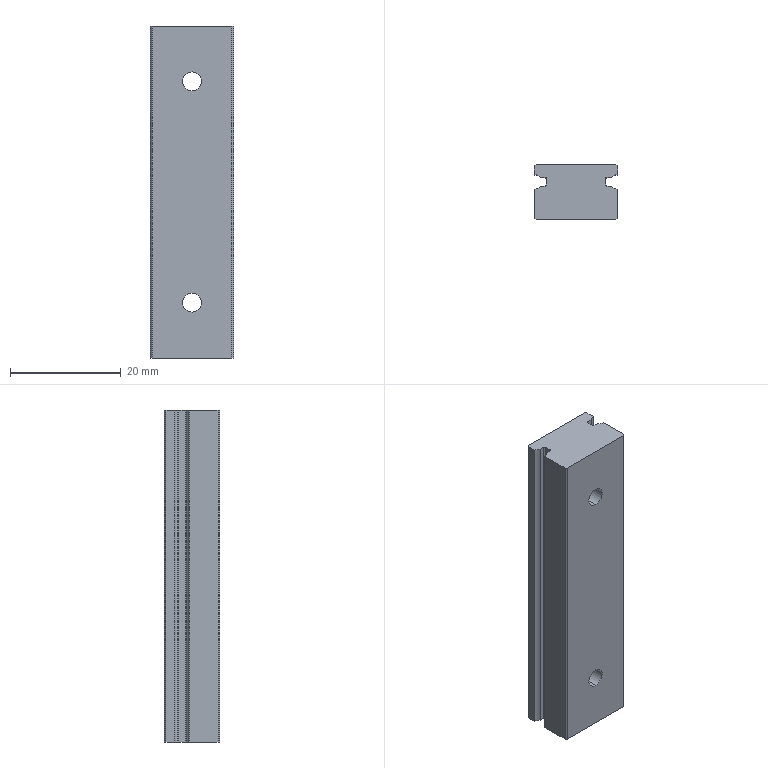Part | SolidWorks | features 3DProfileFeature 1, Extrusion 1, HoleWzd 1, LPattern 1 | 1 solid | 36 faces | box 15 x 10 x 60 mm | volume 8184 mm3 | plane 20 | cylinder 16 | commonest cylinder face diameters 0.4 x4 2.64 x4 3.4 x4 6 x4
STEP:
#1=CARTESIAN_POINT('',(0.,6.6,-23.));
#2=VERTEX_POINT('',#1);
#3=CARTESIAN_POINT('',(0.,6.6,-17.));
#4=VERTEX_POINT('',#3);
#5=CARTESIAN_POINT('',(0.,6.6,-20.));
#6=DIRECTION('',(0.,1.,0.));
#7=DIRECTION('',(0.,0.,1.));
#8=AXIS2_PLACEMENT_3D('',#5,#6,#7);
#9=CIRCLE('',#8,3.);
#10=EDGE_CURVE('',#2,#4,#9,.T.);
#11=ORIENTED_EDGE('',*,*,#10,.F.);
#12=CARTESIAN_POINT('',(0.,10.,-23.));
#13=VERTEX_POINT('',#12);
#14=CARTESIAN_POINT('',(0.,10.,-23.));
#15=DIRECTION('',(0.,1.,0.));
#16=VECTOR('',#15,1000.);
#17=LINE('',#14,#16);
#18=EDGE_CURVE('',#2,#13,#17,.T.);
#19=ORIENTED_EDGE('',*,*,#18,.T.);
#20=CARTESIAN_POINT('',(0.,10.,-17.));
#21=VERTEX_POINT('',#20);
#22=CARTESIAN_POINT('',(0.,10.,-20.));
#23=DIRECTION('',(0.,1.,0.));
#24=DIRECTION('',(0.,0.,1.));
#25=AXIS2_PLACEMENT_3D('',#22,#23,#24);
#26=CIRCLE('',#25,3.);
#27=EDGE_CURVE('',#13,#21,#26,.T.);
#28=ORIENTED_EDGE('',*,*,#27,.T.);
#29=CARTESIAN_POINT('',(0.,10.,-17.));
#30=DIRECTION('',(0.,1.,0.));
#31=VECTOR('',#30,1000.);
#32=LINE('',#29,#31);
#33=EDGE_CURVE('',#4,#21,#32,.T.);
#34=ORIENTED_EDGE('',*,*,#33,.F.);
#35=EDGE_LOOP('',(#11,#19,#28,#34));
#36=FACE_OUTER_BOUND('',#35,.T.);
#37=CARTESIAN_POINT('',(0.,10.,-20.));
#38=DIRECTION('',(0.,1.,0.));
#39=DIRECTION('',(0.,0.,1.));
#40=AXIS2_PLACEMENT_3D('',#37,#38,#39);
#41=CYLINDRICAL_SURFACE('',#40,3.);
#42=ADVANCED_FACE('',(#36),#41,.F.);
#43=CARTESIAN_POINT('',(0.,0.,-21.7));
#44=VERTEX_POINT('',#43);
#45=CARTESIAN_POINT('',(0.,0.,-18.3));
#46=VERTEX_POINT('',#45);
#47=CARTESIAN_POINT('',(0.,0.,-20.));
#48=DIRECTION('',(0.,1.,0.));
#49=DIRECTION('',(0.,0.,1.));
#50=AXIS2_PLACEMENT_3D('',#47,#48,#49);
#51=CIRCLE('',#50,1.7);
#52=EDGE_CURVE('',#44,#46,#51,.T.);
#53=ORIENTED_EDGE('',*,*,#52,.F.);
#54=CARTESIAN_POINT('',(0.,6.6,-21.7));
#55=VERTEX_POINT('',#54);
#56=CARTESIAN_POINT('',(0.,10.,-21.7));
#57=DIRECTION('',(0.,1.,0.));
#58=VECTOR('',#57,1000.);
#59=LINE('',#56,#58);
#60=EDGE_CURVE('',#44,#55,#59,.T.);
#61=ORIENTED_EDGE('',*,*,#60,.T.);
#62=CARTESIAN_POINT('',(0.,6.6,-18.3));
#63=VERTEX_POINT('',#62);
#64=CARTESIAN_POINT('',(0.,6.6,-20.));
#65=DIRECTION('',(0.,1.,0.));
#66=DIRECTION('',(0.,0.,1.));
#67=AXIS2_PLACEMENT_3D('',#64,#65,#66);
#68=CIRCLE('',#67,1.7);
#69=EDGE_CURVE('',#55,#63,#68,.T.);
#70=ORIENTED_EDGE('',*,*,#69,.T.);
#71=CARTESIAN_POINT('',(0.,10.,-18.3));
#72=DIRECTION('',(0.,1.,0.));
#73=VECTOR('',#72,1000.);
#74=LINE('',#71,#73);
#75=EDGE_CURVE('',#46,#63,#74,.T.);
#76=ORIENTED_EDGE('',*,*,#75,.F.);
#77=EDGE_LOOP('',(#53,#61,#70,#76));
#78=FACE_OUTER_BOUND('',#77,.T.);
#79=CARTESIAN_POINT('',(0.,10.,-20.));
#80=DIRECTION('',(0.,1.,0.));
#81=DIRECTION('',(0.,0.,1.));
#82=AXIS2_PLACEMENT_3D('',#79,#80,#81);
#83=CYLINDRICAL_SURFACE('',#82,1.7);
#84=ADVANCED_FACE('',(#78),#83,.F.);
#85=CARTESIAN_POINT('',(0.,6.6,17.));
#86=VERTEX_POINT('',#85);
#87=CARTESIAN_POINT('',(0.,6.6,23.));
#88=VERTEX_POINT('',#87);
#89=CARTESIAN_POINT('',(0.,6.6,20.));
#90=DIRECTION('',(0.,1.,0.));
#91=DIRECTION('',(0.,0.,1.));
#92=AXIS2_PLACEMENT_3D('',#89,#90,#91);
#93=CIRCLE('',#92,3.);
#94=EDGE_CURVE('',#86,#88,#93,.T.);
#95=ORIENTED_EDGE('',*,*,#94,.F.);
#96=CARTESIAN_POINT('',(0.,10.,17.));
#97=VERTEX_POINT('',#96);
#98=CARTESIAN_POINT('',(0.,10.,17.));
#99=DIRECTION('',(0.,1.,0.));
#100=VECTOR('',#99,1000.);
#101=LINE('',#98,#100);
#102=EDGE_CURVE('',#86,#97,#101,.T.);
#103=ORIENTED_EDGE('',*,*,#102,.T.);
#104=CARTESIAN_POINT('',(0.,10.,23.));
#105=VERTEX_POINT('',#104);
#106=CARTESIAN_POINT('',(0.,10.,20.));
#107=DIRECTION('',(0.,1.,0.));
#108=DIRECTION('',(0.,0.,1.));
#109=AXIS2_PLACEMENT_3D('',#106,#107,#108);
#110=CIRCLE('',#109,3.);
#111=EDGE_CURVE('',#97,#105,#110,.T.);
#112=ORIENTED_EDGE('',*,*,#111,.T.);
#113=CARTESIAN_POINT('',(0.,10.,23.));
#114=DIRECTION('',(0.,1.,0.));
#115=VECTOR('',#114,1000.);
#116=LINE('',#113,#115);
#117=EDGE_CURVE('',#88,#105,#116,.T.);
#118=ORIENTED_EDGE('',*,*,#117,.F.);
#119=EDGE_LOOP('',(#95,#103,#112,#118));
#120=FACE_OUTER_BOUND('',#119,.T.);
#121=CARTESIAN_POINT('',(0.,10.,20.));
#122=DIRECTION('',(0.,1.,0.));
#123=DIRECTION('',(0.,0.,1.));
#124=AXIS2_PLACEMENT_3D('',#121,#122,#123);
#125=CYLINDRICAL_SURFACE('',#124,3.);
#126=ADVANCED_FACE('',(#120),#125,.F.);
#127=CARTESIAN_POINT('',(0.,0.,18.3));
#128=VERTEX_POINT('',#127);
#129=CARTESIAN_POINT('',(0.,0.,21.7));
#130=VERTEX_POINT('',#129);
#131=CARTESIAN_POINT('',(0.,0.,20.));
#132=DIRECTION('',(0.,1.,0.));
#133=DIRECTION('',(0.,0.,1.));
#134=AXIS2_PLACEMENT_3D('',#131,#132,#133);
#135=CIRCLE('',#134,1.7);
#136=EDGE_CURVE('',#128,#130,#135,.T.);
#137=ORIENTED_EDGE('',*,*,#136,.F.);
#138=CARTESIAN_POINT('',(0.,6.6,18.3));
#139=VERTEX_POINT('',#138);
#140=CARTESIAN_POINT('',(0.,10.,18.3));
#141=DIRECTION('',(0.,1.,0.));
#142=VECTOR('',#141,1000.);
#143=LINE('',#140,#142);
#144=EDGE_CURVE('',#128,#139,#143,.T.);
#145=ORIENTED_EDGE('',*,*,#144,.T.);
#146=CARTESIAN_POINT('',(0.,6.6,21.7));
#147=VERTEX_POINT('',#146);
#148=CARTESIAN_POINT('',(0.,6.6,20.));
#149=DIRECTION('',(0.,1.,0.));
#150=DIRECTION('',(0.,0.,1.));
#151=AXIS2_PLACEMENT_3D('',#148,#149,#150);
#152=CIRCLE('',#151,1.7);
#153=EDGE_CURVE('',#139,#147,#152,.T.);
#154=ORIENTED_EDGE('',*,*,#153,.T.);
#155=CARTESIAN_POINT('',(0.,10.,21.7));
#156=DIRECTION('',(0.,1.,0.));
#157=VECTOR('',#156,1000.);
#158=LINE('',#155,#157);
#159=EDGE_CURVE('',#130,#147,#158,.T.);
#160=ORIENTED_EDGE('',*,*,#159,.F.);
#161=EDGE_LOOP('',(#137,#145,#154,#160));
#162=FACE_OUTER_BOUND('',#161,.T.);
#163=CARTESIAN_POINT('',(0.,10.,20.));
#164=DIRECTION('',(0.,1.,0.));
#165=DIRECTION('',(0.,0.,1.));
#166=AXIS2_PLACEMENT_3D('',#163,#164,#165);
#167=CYLINDRICAL_SURFACE('',#166,1.7);
#168=ADVANCED_FACE('',(#162),#167,.F.);
#169=CARTESIAN_POINT('',(7.5,8.12,-30.));
#170=VERTEX_POINT('',#169);
#171=CARTESIAN_POINT('',(7.5,9.7,-30.));
#172=VERTEX_POINT('',#171);
#173=CARTESIAN_POINT('',(7.5,8.12,-30.));
#174=DIRECTION('',(0.,1.,0.));
#175=VECTOR('',#174,1000.);
#176=LINE('',#173,#175);
#177=EDGE_CURVE('',#170,#172,#176,.T.);
#178=ORIENTED_EDGE('',*,*,#177,.T.);
#179=CARTESIAN_POINT('',(7.5,9.7,30.));
#180=VERTEX_POINT('',#179);
#181=CARTESIAN_POINT('',(7.5,9.7,30.));
#182=DIRECTION('',(0.,0.,-1.));
#183=VECTOR('',#182,1000.);
#184=LINE('',#181,#183);
#185=EDGE_CURVE('',#180,#172,#184,.T.);
#186=ORIENTED_EDGE('',*,*,#185,.F.);
#187=CARTESIAN_POINT('',(7.5,8.12,30.));
#188=VERTEX_POINT('',#187);
#189=CARTESIAN_POINT('',(7.5,8.12,30.));
#190=DIRECTION('',(0.,1.,0.));
#191=VECTOR('',#190,1000.);
#192=LINE('',#189,#191);
#193=EDGE_CURVE('',#188,#180,#192,.T.);
#194=ORIENTED_EDGE('',*,*,#193,.F.);
#195=CARTESIAN_POINT('',(7.5,8.12,30.));
#196=DIRECTION('',(0.,0.,-1.));
#197=VECTOR('',#196,1000.);
#198=LINE('',#195,#197);
#199=EDGE_CURVE('',#188,#170,#198,.T.);
#200=ORIENTED_EDGE('',*,*,#199,.T.);
#201=EDGE_LOOP('',(#178,#186,#194,#200));
#202=FACE_OUTER_BOUND('',#201,.T.);
#203=CARTESIAN_POINT('',(7.5,8.12,30.));
#204=DIRECTION('',(-1.,0.,0.));
#205=DIRECTION('',(0.,0.,1.));
#206=AXIS2_PLACEMENT_3D('',#203,#204,#205);
#207=PLANE('',#206);
#208=ADVANCED_FACE('',(#202),#207,.F.);
#209=CARTESIAN_POINT('',(7.2,10.,-30.));
#210=VERTEX_POINT('',#209);
#211=CARTESIAN_POINT('',(7.5,9.7,-30.));
#212=DIRECTION('',(-0.7071,0.7071,0.));
#213=VECTOR('',#212,1000.);
#214=LINE('',#211,#213);
#215=EDGE_CURVE('',#172,#210,#214,.T.);
#216=ORIENTED_EDGE('',*,*,#215,.T.);
#217=CARTESIAN_POINT('',(7.2,10.,30.));
#218=VERTEX_POINT('',#217);
#219=CARTESIAN_POINT('',(7.2,10.,30.));
#220=DIRECTION('',(0.,0.,-1.));
#221=VECTOR('',#220,1000.);
#222=LINE('',#219,#221);
#223=EDGE_CURVE('',#218,#210,#222,.T.);
#224=ORIENTED_EDGE('',*,*,#223,.F.);
#225=CARTESIAN_POINT('',(7.5,9.7,30.));
#226=DIRECTION('',(-0.7071,0.7071,0.));
#227=VECTOR('',#226,1000.);
#228=LINE('',#225,#227);
#229=EDGE_CURVE('',#180,#218,#228,.T.);
#230=ORIENTED_EDGE('',*,*,#229,.F.);
#231=ORIENTED_EDGE('',*,*,#185,.T.);
#232=EDGE_LOOP('',(#216,#224,#230,#231));
#233=FACE_OUTER_BOUND('',#232,.T.);
#234=CARTESIAN_POINT('',(7.5,9.7,30.));
#235=DIRECTION('',(-0.7071,-0.7071,0.));
#236=DIRECTION('',(0.7071,-0.7071,0.));
#237=AXIS2_PLACEMENT_3D('',#234,#235,#236);
#238=PLANE('',#237);
#239=ADVANCED_FACE('',(#233),#238,.F.);
#240=CARTESIAN_POINT('',(0.,10.,-20.));
#241=DIRECTION('',(0.,1.,0.));
#242=DIRECTION('',(0.,0.,1.));
#243=AXIS2_PLACEMENT_3D('',#240,#241,#242);
#244=CIRCLE('',#243,3.);
#245=EDGE_CURVE('',#21,#13,#244,.T.);
#246=ORIENTED_EDGE('',*,*,#245,.F.);
#247=ORIENTED_EDGE('',*,*,#27,.F.);
#248=EDGE_LOOP('',(#246,#247));
#249=FACE_BOUND('',#248,.T.);
#250=CARTESIAN_POINT('',(0.,10.,20.));
#251=DIRECTION('',(0.,1.,0.));
#252=DIRECTION('',(0.,0.,1.));
#253=AXIS2_PLACEMENT_3D('',#250,#251,#252);
#254=CIRCLE('',#253,3.);
#255=EDGE_CURVE('',#105,#97,#254,.T.);
#256=ORIENTED_EDGE('',*,*,#255,.F.);
#257=ORIENTED_EDGE('',*,*,#111,.F.);
#258=EDGE_LOOP('',(#256,#257));
#259=FACE_BOUND('',#258,.T.);
#260=CARTESIAN_POINT('',(-7.2,10.,-30.));
#261=VERTEX_POINT('',#260);
#262=CARTESIAN_POINT('',(7.2,10.,-30.));
#263=DIRECTION('',(-1.,0.,0.));
#264=VECTOR('',#263,1000.);
#265=LINE('',#262,#264);
#266=EDGE_CURVE('',#210,#261,#265,.T.);
#267=ORIENTED_EDGE('',*,*,#266,.T.);
#268=CARTESIAN_POINT('',(-7.2,10.,30.));
#269=VERTEX_POINT('',#268);
#270=CARTESIAN_POINT('',(-7.2,10.,30.));
#271=DIRECTION('',(0.,0.,-1.));
#272=VECTOR('',#271,1000.);
#273=LINE('',#270,#272);
#274=EDGE_CURVE('',#269,#261,#273,.T.);
#275=ORIENTED_EDGE('',*,*,#274,.F.);
#276=CARTESIAN_POINT('',(7.2,10.,30.));
#277=DIRECTION('',(-1.,0.,0.));
#278=VECTOR('',#277,1000.);
#279=LINE('',#276,#278);
#280=EDGE_CURVE('',#218,#269,#279,.T.);
#281=ORIENTED_EDGE('',*,*,#280,.F.);
#282=ORIENTED_EDGE('',*,*,#223,.T.);
#283=EDGE_LOOP('',(#267,#275,#281,#282));
#284=FACE_OUTER_BOUND('',#283,.T.);
#285=CARTESIAN_POINT('',(7.2,10.,30.));
#286=DIRECTION('',(0.,-1.,0.));
#287=DIRECTION('',(0.,0.,-1.));
#288=AXIS2_PLACEMENT_3D('',#285,#286,#287);
#289=PLANE('',#288);
#290=ADVANCED_FACE('',(#249,#259,#284),#289,.F.);
#291=CARTESIAN_POINT('',(-7.5,9.7,-30.));
#292=VERTEX_POINT('',#291);
#293=CARTESIAN_POINT('',(-7.2,10.,-30.));
#294=DIRECTION('',(-0.7071,-0.7071,0.));
#295=VECTOR('',#294,1000.);
#296=LINE('',#293,#295);
#297=EDGE_CURVE('',#261,#292,#296,.T.);
#298=ORIENTED_EDGE('',*,*,#297,.T.);
#299=CARTESIAN_POINT('',(-7.5,9.7,30.));
#300=VERTEX_POINT('',#299);
#301=CARTESIAN_POINT('',(-7.5,9.7,30.));
#302=DIRECTION('',(0.,0.,-1.));
#303=VECTOR('',#302,1000.);
#304=LINE('',#301,#303);
#305=EDGE_CURVE('',#300,#292,#304,.T.);
#306=ORIENTED_EDGE('',*,*,#305,.F.);
#307=CARTESIAN_POINT('',(-7.2,10.,30.));
#308=DIRECTION('',(-0.7071,-0.7071,0.));
#309=VECTOR('',#308,1000.);
#310=LINE('',#307,#309);
#311=EDGE_CURVE('',#269,#300,#310,.T.);
#312=ORIENTED_EDGE('',*,*,#311,.F.);
#313=ORIENTED_EDGE('',*,*,#274,.T.);
#314=EDGE_LOOP('',(#298,#306,#312,#313));
#315=FACE_OUTER_BOUND('',#314,.T.);
#316=CARTESIAN_POINT('',(-7.2,10.,30.));
#317=DIRECTION('',(0.7071,-0.7071,0.));
#318=DIRECTION('',(0.7071,0.7071,0.));
#319=AXIS2_PLACEMENT_3D('',#316,#317,#318);
#320=PLANE('',#319);
#321=ADVANCED_FACE('',(#315),#320,.F.);
#322=CARTESIAN_POINT('',(-7.5,8.12,-30.));
#323=VERTEX_POINT('',#322);
#324=CARTESIAN_POINT('',(-7.5,9.7,-30.));
#325=DIRECTION('',(0.,-1.,0.));
#326=VECTOR('',#325,1000.);
#327=LINE('',#324,#326);
#328=EDGE_CURVE('',#292,#323,#327,.T.);
#329=ORIENTED_EDGE('',*,*,#328,.T.);
#330=CARTESIAN_POINT('',(-7.5,8.12,30.));
#331=VERTEX_POINT('',#330);
#332=CARTESIAN_POINT('',(-7.5,8.12,30.));
#333=DIRECTION('',(0.,0.,-1.));
#334=VECTOR('',#333,1000.);
#335=LINE('',#332,#334);
#336=EDGE_CURVE('',#331,#323,#335,.T.);
#337=ORIENTED_EDGE('',*,*,#336,.F.);
#338=CARTESIAN_POINT('',(-7.5,9.7,30.));
#339=DIRECTION('',(0.,-1.,0.));
#340=VECTOR('',#339,1000.);
#341=LINE('',#338,#340);
#342=EDGE_CURVE('',#300,#331,#341,.T.);
#343=ORIENTED_EDGE('',*,*,#342,.F.);
#344=ORIENTED_EDGE('',*,*,#305,.T.);
#345=EDGE_LOOP('',(#329,#337,#343,#344));
#346=FACE_OUTER_BOUND('',#345,.T.);
#347=CARTESIAN_POINT('',(-7.5,9.7,30.));
#348=DIRECTION('',(1.,0.,0.));
#349=DIRECTION('',(0.,0.,-1.));
#350=AXIS2_PLACEMENT_3D('',#347,#348,#349);
#351=PLANE('',#350);
#352=ADVANCED_FACE('',(#346),#351,.F.);
#353=CARTESIAN_POINT('',(-6.45,7.6,-30.));
#354=VERTEX_POINT('',#353);
#355=CARTESIAN_POINT('',(-7.5,6.8,-30.));
#356=DIRECTION('',(0.,0.,-1.));
#357=DIRECTION('',(1.,0.,0.));
#358=AXIS2_PLACEMENT_3D('',#355,#356,#357);
#359=CIRCLE('',#358,1.32);
#360=EDGE_CURVE('',#323,#354,#359,.T.);
#361=ORIENTED_EDGE('',*,*,#360,.T.);
#362=CARTESIAN_POINT('',(-6.45,7.6,30.));
#363=VERTEX_POINT('',#362);
#364=CARTESIAN_POINT('',(-6.45,7.6,30.));
#365=DIRECTION('',(0.,0.,-1.));
#366=VECTOR('',#365,1000.);
#367=LINE('',#364,#366);
#368=EDGE_CURVE('',#363,#354,#367,.T.);
#369=ORIENTED_EDGE('',*,*,#368,.F.);
#370=CARTESIAN_POINT('',(-7.5,6.8,30.));
#371=DIRECTION('',(0.,0.,-1.));
#372=DIRECTION('',(1.,0.,0.));
#373=AXIS2_PLACEMENT_3D('',#370,#371,#372);
#374=CIRCLE('',#373,1.32);
#375=EDGE_CURVE('',#331,#363,#374,.T.);
#376=ORIENTED_EDGE('',*,*,#375,.F.);
#377=ORIENTED_EDGE('',*,*,#336,.T.);
#378=EDGE_LOOP('',(#361,#369,#376,#377));
#379=FACE_OUTER_BOUND('',#378,.T.);
#380=CARTESIAN_POINT('',(-7.5,6.8,30.));
#381=DIRECTION('',(0.,0.,-1.));
#382=DIRECTION('',(-1.,0.,0.));
#383=AXIS2_PLACEMENT_3D('',#380,#381,#382);
#384=CYLINDRICAL_SURFACE('',#383,1.32);
#385=ADVANCED_FACE('',(#379),#384,.F.);
#386=CARTESIAN_POINT('',(-5.6,7.6,-30.));
#387=VERTEX_POINT('',#386);
#388=CARTESIAN_POINT('',(-6.45,7.6,-30.));
#389=DIRECTION('',(1.,0.,0.));
#390=VECTOR('',#389,1000.);
#391=LINE('',#388,#390);
#392=EDGE_CURVE('',#354,#387,#391,.T.);
#393=ORIENTED_EDGE('',*,*,#392,.T.);
#394=CARTESIAN_POINT('',(-5.6,7.6,30.));
#395=VERTEX_POINT('',#394);
#396=CARTESIAN_POINT('',(-5.6,7.6,30.));
#397=DIRECTION('',(0.,0.,-1.));
#398=VECTOR('',#397,1000.);
#399=LINE('',#396,#398);
#400=EDGE_CURVE('',#395,#387,#399,.T.);
#401=ORIENTED_EDGE('',*,*,#400,.F.);
#402=CARTESIAN_POINT('',(-6.45,7.6,30.));
#403=DIRECTION('',(1.,0.,0.));
#404=VECTOR('',#403,1000.);
#405=LINE('',#402,#404);
#406=EDGE_CURVE('',#363,#395,#405,.T.);
#407=ORIENTED_EDGE('',*,*,#406,.F.);
#408=ORIENTED_EDGE('',*,*,#368,.T.);
#409=EDGE_LOOP('',(#393,#401,#407,#408));
#410=FACE_OUTER_BOUND('',#409,.T.);
#411=CARTESIAN_POINT('',(-6.45,7.6,30.));
#412=DIRECTION('',(0.,1.,0.));
#413=DIRECTION('',(0.,0.,1.));
#414=AXIS2_PLACEMENT_3D('',#411,#412,#413);
#415=PLANE('',#414);
#416=ADVANCED_FACE('',(#410),#415,.F.);
#417=CARTESIAN_POINT('',(-5.4,7.4,-30.));
#418=VERTEX_POINT('',#417);
#419=CARTESIAN_POINT('',(-5.6,7.4,-30.));
#420=DIRECTION('',(0.,0.,-1.));
#421=DIRECTION('',(1.,0.,0.));
#422=AXIS2_PLACEMENT_3D('',#419,#420,#421);
#423=CIRCLE('',#422,0.2);
#424=EDGE_CURVE('',#387,#418,#423,.T.);
#425=ORIENTED_EDGE('',*,*,#424,.T.);
#426=CARTESIAN_POINT('',(-5.4,7.4,30.));
#427=VERTEX_POINT('',#426);
#428=CARTESIAN_POINT('',(-5.4,7.4,30.));
#429=DIRECTION('',(0.,0.,-1.));
#430=VECTOR('',#429,1000.);
#431=LINE('',#428,#430);
#432=EDGE_CURVE('',#427,#418,#431,.T.);
#433=ORIENTED_EDGE('',*,*,#432,.F.);
#434=CARTESIAN_POINT('',(-5.6,7.4,30.));
#435=DIRECTION('',(0.,0.,-1.));
#436=DIRECTION('',(1.,0.,0.));
#437=AXIS2_PLACEMENT_3D('',#434,#435,#436);
#438=CIRCLE('',#437,0.2);
#439=EDGE_CURVE('',#395,#427,#438,.T.);
#440=ORIENTED_EDGE('',*,*,#439,.F.);
#441=ORIENTED_EDGE('',*,*,#400,.T.);
#442=EDGE_LOOP('',(#425,#433,#440,#441));
#443=FACE_OUTER_BOUND('',#442,.T.);
#444=CARTESIAN_POINT('',(-5.6,7.4,30.));
#445=DIRECTION('',(0.,0.,-1.));
#446=DIRECTION('',(-1.,0.,0.));
#447=AXIS2_PLACEMENT_3D('',#444,#445,#446);
#448=CYLINDRICAL_SURFACE('',#447,0.2);
#449=ADVANCED_FACE('',(#443),#448,.F.);
#450=CARTESIAN_POINT('',(-5.4,6.2,-30.));
#451=VERTEX_POINT('',#450);
#452=CARTESIAN_POINT('',(-5.4,7.4,-30.));
#453=DIRECTION('',(0.,-1.,0.));
#454=VECTOR('',#453,1000.);
#455=LINE('',#452,#454);
#456=EDGE_CURVE('',#418,#451,#455,.T.);
#457=ORIENTED_EDGE('',*,*,#456,.T.);
#458=CARTESIAN_POINT('',(-5.4,6.2,30.));
#459=VERTEX_POINT('',#458);
#460=CARTESIAN_POINT('',(-5.4,6.2,30.));
#461=DIRECTION('',(0.,0.,-1.));
#462=VECTOR('',#461,1000.);
#463=LINE('',#460,#462);
#464=EDGE_CURVE('',#459,#451,#463,.T.);
#465=ORIENTED_EDGE('',*,*,#464,.F.);
#466=CARTESIAN_POINT('',(-5.4,7.4,30.));
#467=DIRECTION('',(0.,-1.,0.));
#468=VECTOR('',#467,1000.);
#469=LINE('',#466,#468);
#470=EDGE_CURVE('',#427,#459,#469,.T.);
#471=ORIENTED_EDGE('',*,*,#470,.F.);
#472=ORIENTED_EDGE('',*,*,#432,.T.);
#473=EDGE_LOOP('',(#457,#465,#471,#472));
#474=FACE_OUTER_BOUND('',#473,.T.);
#475=CARTESIAN_POINT('',(-5.4,7.4,30.));
#476=DIRECTION('',(1.,0.,0.));
#477=DIRECTION('',(0.,0.,-1.));
#478=AXIS2_PLACEMENT_3D('',#475,#476,#477);
#479=PLANE('',#478);
#480=ADVANCED_FACE('',(#474),#479,.F.);
#481=CARTESIAN_POINT('',(-5.6,6.,-30.));
#482=VERTEX_POINT('',#481);
#483=CARTESIAN_POINT('',(-5.6,6.2,-30.));
#484=DIRECTION('',(0.,0.,-1.));
#485=DIRECTION('',(1.,0.,0.));
#486=AXIS2_PLACEMENT_3D('',#483,#484,#485);
#487=CIRCLE('',#486,0.2);
#488=EDGE_CURVE('',#451,#482,#487,.T.);
#489=ORIENTED_EDGE('',*,*,#488,.T.);
#490=CARTESIAN_POINT('',(-5.6,6.,30.));
#491=VERTEX_POINT('',#490);
#492=CARTESIAN_POINT('',(-5.6,6.,30.));
#493=DIRECTION('',(0.,0.,-1.));
#494=VECTOR('',#493,1000.);
#495=LINE('',#492,#494);
#496=EDGE_CURVE('',#491,#482,#495,.T.);
#497=ORIENTED_EDGE('',*,*,#496,.F.);
#498=CARTESIAN_POINT('',(-5.6,6.2,30.));
#499=DIRECTION('',(0.,0.,-1.));
#500=DIRECTION('',(1.,0.,0.));
#501=AXIS2_PLACEMENT_3D('',#498,#499,#500);
#502=CIRCLE('',#501,0.2);
#503=EDGE_CURVE('',#459,#491,#502,.T.);
#504=ORIENTED_EDGE('',*,*,#503,.F.);
#505=ORIENTED_EDGE('',*,*,#464,.T.);
#506=EDGE_LOOP('',(#489,#497,#504,#505));
#507=FACE_OUTER_BOUND('',#506,.T.);
#508=CARTESIAN_POINT('',(-5.6,6.2,30.));
#509=DIRECTION('',(0.,0.,-1.));
#510=DIRECTION('',(-1.,0.,0.));
#511=AXIS2_PLACEMENT_3D('',#508,#509,#510);
#512=CYLINDRICAL_SURFACE('',#511,0.2);
#513=ADVANCED_FACE('',(#507),#512,.F.);
#514=CARTESIAN_POINT('',(-6.45,6.,-30.));
#515=VERTEX_POINT('',#514);
#516=CARTESIAN_POINT('',(-5.6,6.,-30.));
#517=DIRECTION('',(-1.,0.,0.));
#518=VECTOR('',#517,1000.);
#519=LINE('',#516,#518);
#520=EDGE_CURVE('',#482,#515,#519,.T.);
#521=ORIENTED_EDGE('',*,*,#520,.T.);
#522=CARTESIAN_POINT('',(-6.45,6.,30.));
#523=VERTEX_POINT('',#522);
#524=CARTESIAN_POINT('',(-6.45,6.,30.));
#525=DIRECTION('',(0.,0.,-1.));
#526=VECTOR('',#525,1000.);
#527=LINE('',#524,#526);
#528=EDGE_CURVE('',#523,#515,#527,.T.);
#529=ORIENTED_EDGE('',*,*,#528,.F.);
#530=CARTESIAN_POINT('',(-5.6,6.,30.));
#531=DIRECTION('',(-1.,0.,0.));
#532=VECTOR('',#531,1000.);
#533=LINE('',#530,#532);
#534=EDGE_CURVE('',#491,#523,#533,.T.);
#535=ORIENTED_EDGE('',*,*,#534,.F.);
#536=ORIENTED_EDGE('',*,*,#496,.T.);
#537=EDGE_LOOP('',(#521,#529,#535,#536));
#538=FACE_OUTER_BOUND('',#537,.T.);
#539=CARTESIAN_POINT('',(-5.6,6.,30.));
#540=DIRECTION('',(0.,-1.,0.));
#541=DIRECTION('',(0.,0.,-1.));
#542=AXIS2_PLACEMENT_3D('',#539,#540,#541);
#543=PLANE('',#542);
#544=ADVANCED_FACE('',(#538),#543,.F.);
#545=CARTESIAN_POINT('',(-7.5,5.48,-30.));
#546=VERTEX_POINT('',#545);
#547=CARTESIAN_POINT('',(-7.5,6.8,-30.));
#548=DIRECTION('',(0.,0.,-1.));
#549=DIRECTION('',(1.,0.,0.));
#550=AXIS2_PLACEMENT_3D('',#547,#548,#549);
#551=CIRCLE('',#550,1.32);
#552=EDGE_CURVE('',#515,#546,#551,.T.);
#553=ORIENTED_EDGE('',*,*,#552,.T.);
#554=CARTESIAN_POINT('',(-7.5,5.48,30.));
#555=VERTEX_POINT('',#554);
#556=CARTESIAN_POINT('',(-7.5,5.48,30.));
#557=DIRECTION('',(0.,0.,-1.));
#558=VECTOR('',#557,1000.);
#559=LINE('',#556,#558);
#560=EDGE_CURVE('',#555,#546,#559,.T.);
#561=ORIENTED_EDGE('',*,*,#560,.F.);
#562=CARTESIAN_POINT('',(-7.5,6.8,30.));
#563=DIRECTION('',(0.,0.,-1.));
#564=DIRECTION('',(1.,0.,0.));
#565=AXIS2_PLACEMENT_3D('',#562,#563,#564);
#566=CIRCLE('',#565,1.32);
#567=EDGE_CURVE('',#523,#555,#566,.T.);
#568=ORIENTED_EDGE('',*,*,#567,.F.);
#569=ORIENTED_EDGE('',*,*,#528,.T.);
#570=EDGE_LOOP('',(#553,#561,#568,#569));
#571=FACE_OUTER_BOUND('',#570,.T.);
#572=CARTESIAN_POINT('',(-7.5,6.8,30.));
#573=DIRECTION('',(0.,0.,-1.));
#574=DIRECTION('',(-1.,0.,0.));
#575=AXIS2_PLACEMENT_3D('',#572,#573,#574);
#576=CYLINDRICAL_SURFACE('',#575,1.32);
#577=ADVANCED_FACE('',(#571),#576,.F.);
#578=CARTESIAN_POINT('',(-7.5,0.3,-30.));
#579=VERTEX_POINT('',#578);
#580=CARTESIAN_POINT('',(-7.5,5.48,-30.));
#581=DIRECTION('',(0.,-1.,0.));
#582=VECTOR('',#581,1000.);
#583=LINE('',#580,#582);
#584=EDGE_CURVE('',#546,#579,#583,.T.);
#585=ORIENTED_EDGE('',*,*,#584,.T.);
#586=CARTESIAN_POINT('',(-7.5,0.3,30.));
#587=VERTEX_POINT('',#586);
#588=CARTESIAN_POINT('',(-7.5,0.3,30.));
#589=DIRECTION('',(0.,0.,-1.));
#590=VECTOR('',#589,1000.);
#591=LINE('',#588,#590);
#592=EDGE_CURVE('',#587,#579,#591,.T.);
#593=ORIENTED_EDGE('',*,*,#592,.F.);
#594=CARTESIAN_POINT('',(-7.5,5.48,30.));
#595=DIRECTION('',(0.,-1.,0.));
#596=VECTOR('',#595,1000.);
#597=LINE('',#594,#596);
#598=EDGE_CURVE('',#555,#587,#597,.T.);
#599=ORIENTED_EDGE('',*,*,#598,.F.);
#600=ORIENTED_EDGE('',*,*,#560,.T.);
#601=EDGE_LOOP('',(#585,#593,#599,#600));
#602=FACE_OUTER_BOUND('',#601,.T.);
#603=CARTESIAN_POINT('',(-7.5,5.48,30.));
#604=DIRECTION('',(1.,0.,0.));
#605=DIRECTION('',(0.,0.,-1.));
#606=AXIS2_PLACEMENT_3D('',#603,#604,#605);
#607=PLANE('',#606);
#608=ADVANCED_FACE('',(#602),#607,.F.);
#609=CARTESIAN_POINT('',(-7.2,0.,-30.));
#610=VERTEX_POINT('',#609);
#611=CARTESIAN_POINT('',(-7.5,0.3,-30.));
#612=DIRECTION('',(0.7071,-0.7071,0.));
#613=VECTOR('',#612,1000.);
#614=LINE('',#611,#613);
#615=EDGE_CURVE('',#579,#610,#614,.T.);
#616=ORIENTED_EDGE('',*,*,#615,.T.);
#617=CARTESIAN_POINT('',(-7.2,0.,30.));
#618=VERTEX_POINT('',#617);
#619=CARTESIAN_POINT('',(-7.2,0.,30.));
#620=DIRECTION('',(0.,0.,-1.));
#621=VECTOR('',#620,1000.);
#622=LINE('',#619,#621);
#623=EDGE_CURVE('',#618,#610,#622,.T.);
#624=ORIENTED_EDGE('',*,*,#623,.F.);
#625=CARTESIAN_POINT('',(-7.5,0.3,30.));
#626=DIRECTION('',(0.7071,-0.7071,0.));
#627=VECTOR('',#626,1000.);
#628=LINE('',#625,#627);
#629=EDGE_CURVE('',#587,#618,#628,.T.);
#630=ORIENTED_EDGE('',*,*,#629,.F.);
#631=ORIENTED_EDGE('',*,*,#592,.T.);
#632=EDGE_LOOP('',(#616,#624,#630,#631));
#633=FACE_OUTER_BOUND('',#632,.T.);
#634=CARTESIAN_POINT('',(-7.5,0.3,30.));
#635=DIRECTION('',(0.7071,0.7071,0.));
#636=DIRECTION('',(-0.7071,0.7071,0.));
#637=AXIS2_PLACEMENT_3D('',#634,#635,#636);
#638=PLANE('',#637);
#639=ADVANCED_FACE('',(#633),#638,.F.);
#640=CARTESIAN_POINT('',(0.,0.,-20.));
#641=DIRECTION('',(0.,1.,0.));
#642=DIRECTION('',(0.,0.,1.));
#643=AXIS2_PLACEMENT_3D('',#640,#641,#642);
#644=CIRCLE('',#643,1.7);
#645=EDGE_CURVE('',#46,#44,#644,.T.);
#646=ORIENTED_EDGE('',*,*,#645,.T.);
#647=ORIENTED_EDGE('',*,*,#52,.T.);
#648=EDGE_LOOP('',(#646,#647));
#649=FACE_BOUND('',#648,.T.);
#650=CARTESIAN_POINT('',(0.,0.,20.));
#651=DIRECTION('',(0.,1.,0.));
#652=DIRECTION('',(0.,0.,1.));
#653=AXIS2_PLACEMENT_3D('',#650,#651,#652);
#654=CIRCLE('',#653,1.7);
#655=EDGE_CURVE('',#130,#128,#654,.T.);
#656=ORIENTED_EDGE('',*,*,#655,.T.);
#657=ORIENTED_EDGE('',*,*,#136,.T.);
#658=EDGE_LOOP('',(#656,#657));
#659=FACE_BOUND('',#658,.T.);
#660=CARTESIAN_POINT('',(7.2,0.,-30.));
#661=VERTEX_POINT('',#660);
#662=CARTESIAN_POINT('',(-7.2,0.,-30.));
#663=DIRECTION('',(1.,0.,0.));
#664=VECTOR('',#663,1000.);
#665=LINE('',#662,#664);
#666=EDGE_CURVE('',#610,#661,#665,.T.);
#667=ORIENTED_EDGE('',*,*,#666,.T.);
#668=CARTESIAN_POINT('',(7.2,0.,30.));
#669=VERTEX_POINT('',#668);
#670=CARTESIAN_POINT('',(7.2,0.,30.));
#671=DIRECTION('',(0.,0.,-1.));
#672=VECTOR('',#671,1000.);
#673=LINE('',#670,#672);
#674=EDGE_CURVE('',#669,#661,#673,.T.);
#675=ORIENTED_EDGE('',*,*,#674,.F.);
#676=CARTESIAN_POINT('',(-7.2,0.,30.));
#677=DIRECTION('',(1.,0.,0.));
#678=VECTOR('',#677,1000.);
#679=LINE('',#676,#678);
#680=EDGE_CURVE('',#618,#669,#679,.T.);
#681=ORIENTED_EDGE('',*,*,#680,.F.);
#682=ORIENTED_EDGE('',*,*,#623,.T.);
#683=EDGE_LOOP('',(#667,#675,#681,#682));
#684=FACE_OUTER_BOUND('',#683,.T.);
#685=CARTESIAN_POINT('',(-7.2,0.,30.));
#686=DIRECTION('',(0.,1.,0.));
#687=DIRECTION('',(0.,0.,1.));
#688=AXIS2_PLACEMENT_3D('',#685,#686,#687);
#689=PLANE('',#688);
#690=ADVANCED_FACE('',(#649,#659,#684),#689,.F.);
#691=CARTESIAN_POINT('',(7.5,0.3,-30.));
#692=VERTEX_POINT('',#691);
#693=CARTESIAN_POINT('',(7.2,0.,-30.));
#694=DIRECTION('',(0.7071,0.7071,0.));
#695=VECTOR('',#694,1000.);
#696=LINE('',#693,#695);
#697=EDGE_CURVE('',#661,#692,#696,.T.);
#698=ORIENTED_EDGE('',*,*,#697,.T.);
#699=CARTESIAN_POINT('',(7.5,0.3,30.));
#700=VERTEX_POINT('',#699);
#701=CARTESIAN_POINT('',(7.5,0.3,30.));
#702=DIRECTION('',(0.,0.,-1.));
#703=VECTOR('',#702,1000.);
#704=LINE('',#701,#703);
#705=EDGE_CURVE('',#700,#692,#704,.T.);
#706=ORIENTED_EDGE('',*,*,#705,.F.);
#707=CARTESIAN_POINT('',(7.2,0.,30.));
#708=DIRECTION('',(0.7071,0.7071,0.));
#709=VECTOR('',#708,1000.);
#710=LINE('',#707,#709);
#711=EDGE_CURVE('',#669,#700,#710,.T.);
#712=ORIENTED_EDGE('',*,*,#711,.F.);
#713=ORIENTED_EDGE('',*,*,#674,.T.);
#714=EDGE_LOOP('',(#698,#706,#712,#713));
#715=FACE_OUTER_BOUND('',#714,.T.);
#716=CARTESIAN_POINT('',(7.2,0.,30.));
#717=DIRECTION('',(-0.7071,0.7071,0.));
#718=DIRECTION('',(-0.7071,-0.7071,0.));
#719=AXIS2_PLACEMENT_3D('',#716,#717,#718);
#720=PLANE('',#719);
#721=ADVANCED_FACE('',(#715),#720,.F.);
#722=CARTESIAN_POINT('',(7.5,5.48,-30.));
#723=VERTEX_POINT('',#722);
#724=CARTESIAN_POINT('',(7.5,0.3,-30.));
#725=DIRECTION('',(0.,1.,0.));
#726=VECTOR('',#725,1000.);
#727=LINE('',#724,#726);
#728=EDGE_CURVE('',#692,#723,#727,.T.);
#729=ORIENTED_EDGE('',*,*,#728,.T.);
#730=CARTESIAN_POINT('',(7.5,5.48,30.));
#731=VERTEX_POINT('',#730);
#732=CARTESIAN_POINT('',(7.5,5.48,30.));
#733=DIRECTION('',(0.,0.,-1.));
#734=VECTOR('',#733,1000.);
#735=LINE('',#732,#734);
#736=EDGE_CURVE('',#731,#723,#735,.T.);
#737=ORIENTED_EDGE('',*,*,#736,.F.);
#738=CARTESIAN_POINT('',(7.5,0.3,30.));
#739=DIRECTION('',(0.,1.,0.));
#740=VECTOR('',#739,1000.);
#741=LINE('',#738,#740);
#742=EDGE_CURVE('',#700,#731,#741,.T.);
#743=ORIENTED_EDGE('',*,*,#742,.F.);
#744=ORIENTED_EDGE('',*,*,#705,.T.);
#745=EDGE_LOOP('',(#729,#737,#743,#744));
#746=FACE_OUTER_BOUND('',#745,.T.);
#747=CARTESIAN_POINT('',(7.5,0.3,30.));
#748=DIRECTION('',(-1.,0.,0.));
#749=DIRECTION('',(0.,0.,1.));
#750=AXIS2_PLACEMENT_3D('',#747,#748,#749);
#751=PLANE('',#750);
#752=ADVANCED_FACE('',(#746),#751,.F.);
#753=CARTESIAN_POINT('',(6.45,6.,-30.));
#754=VERTEX_POINT('',#753);
#755=CARTESIAN_POINT('',(7.5,6.8,-30.));
#756=DIRECTION('',(0.,0.,-1.));
#757=DIRECTION('',(1.,0.,0.));
#758=AXIS2_PLACEMENT_3D('',#755,#756,#757);
#759=CIRCLE('',#758,1.32);
#760=EDGE_CURVE('',#723,#754,#759,.T.);
#761=ORIENTED_EDGE('',*,*,#760,.T.);
#762=CARTESIAN_POINT('',(6.45,6.,30.));
#763=VERTEX_POINT('',#762);
#764=CARTESIAN_POINT('',(6.45,6.,30.));
#765=DIRECTION('',(0.,0.,-1.));
#766=VECTOR('',#765,1000.);
#767=LINE('',#764,#766);
#768=EDGE_CURVE('',#763,#754,#767,.T.);
#769=ORIENTED_EDGE('',*,*,#768,.F.);
#770=CARTESIAN_POINT('',(7.5,6.8,30.));
#771=DIRECTION('',(0.,0.,-1.));
#772=DIRECTION('',(1.,0.,0.));
#773=AXIS2_PLACEMENT_3D('',#770,#771,#772);
#774=CIRCLE('',#773,1.32);
#775=EDGE_CURVE('',#731,#763,#774,.T.);
#776=ORIENTED_EDGE('',*,*,#775,.F.);
#777=ORIENTED_EDGE('',*,*,#736,.T.);
#778=EDGE_LOOP('',(#761,#769,#776,#777));
#779=FACE_OUTER_BOUND('',#778,.T.);
#780=CARTESIAN_POINT('',(7.5,6.8,30.));
#781=DIRECTION('',(0.,0.,-1.));
#782=DIRECTION('',(-1.,0.,0.));
#783=AXIS2_PLACEMENT_3D('',#780,#781,#782);
#784=CYLINDRICAL_SURFACE('',#783,1.32);
#785=ADVANCED_FACE('',(#779),#784,.F.);
#786=CARTESIAN_POINT('',(5.6,6.,-30.));
#787=VERTEX_POINT('',#786);
#788=CARTESIAN_POINT('',(6.45,6.,-30.));
#789=DIRECTION('',(-1.,0.,0.));
#790=VECTOR('',#789,1000.);
#791=LINE('',#788,#790);
#792=EDGE_CURVE('',#754,#787,#791,.T.);
#793=ORIENTED_EDGE('',*,*,#792,.T.);
#794=CARTESIAN_POINT('',(5.6,6.,30.));
#795=VERTEX_POINT('',#794);
#796=CARTESIAN_POINT('',(5.6,6.,30.));
#797=DIRECTION('',(0.,0.,-1.));
#798=VECTOR('',#797,1000.);
#799=LINE('',#796,#798);
#800=EDGE_CURVE('',#795,#787,#799,.T.);
#801=ORIENTED_EDGE('',*,*,#800,.F.);
#802=CARTESIAN_POINT('',(6.45,6.,30.));
#803=DIRECTION('',(-1.,0.,0.));
#804=VECTOR('',#803,1000.);
#805=LINE('',#802,#804);
#806=EDGE_CURVE('',#763,#795,#805,.T.);
#807=ORIENTED_EDGE('',*,*,#806,.F.);
#808=ORIENTED_EDGE('',*,*,#768,.T.);
#809=EDGE_LOOP('',(#793,#801,#807,#808));
#810=FACE_OUTER_BOUND('',#809,.T.);
#811=CARTESIAN_POINT('',(6.45,6.,30.));
#812=DIRECTION('',(0.,-1.,0.));
#813=DIRECTION('',(0.,0.,-1.));
#814=AXIS2_PLACEMENT_3D('',#811,#812,#813);
#815=PLANE('',#814);
#816=ADVANCED_FACE('',(#810),#815,.F.);
#817=CARTESIAN_POINT('',(5.4,6.2,-30.));
#818=VERTEX_POINT('',#817);
#819=CARTESIAN_POINT('',(5.6,6.2,-30.));
#820=DIRECTION('',(0.,0.,-1.));
#821=DIRECTION('',(1.,0.,0.));
#822=AXIS2_PLACEMENT_3D('',#819,#820,#821);
#823=CIRCLE('',#822,0.2);
#824=EDGE_CURVE('',#787,#818,#823,.T.);
#825=ORIENTED_EDGE('',*,*,#824,.T.);
#826=CARTESIAN_POINT('',(5.4,6.2,30.));
#827=VERTEX_POINT('',#826);
#828=CARTESIAN_POINT('',(5.4,6.2,30.));
#829=DIRECTION('',(0.,0.,-1.));
#830=VECTOR('',#829,1000.);
#831=LINE('',#828,#830);
#832=EDGE_CURVE('',#827,#818,#831,.T.);
#833=ORIENTED_EDGE('',*,*,#832,.F.);
#834=CARTESIAN_POINT('',(5.6,6.2,30.));
#835=DIRECTION('',(0.,0.,-1.));
#836=DIRECTION('',(1.,0.,0.));
#837=AXIS2_PLACEMENT_3D('',#834,#835,#836);
#838=CIRCLE('',#837,0.2);
#839=EDGE_CURVE('',#795,#827,#838,.T.);
#840=ORIENTED_EDGE('',*,*,#839,.F.);
#841=ORIENTED_EDGE('',*,*,#800,.T.);
#842=EDGE_LOOP('',(#825,#833,#840,#841));
#843=FACE_OUTER_BOUND('',#842,.T.);
#844=CARTESIAN_POINT('',(5.6,6.2,30.));
#845=DIRECTION('',(0.,0.,-1.));
#846=DIRECTION('',(-1.,0.,0.));
#847=AXIS2_PLACEMENT_3D('',#844,#845,#846);
#848=CYLINDRICAL_SURFACE('',#847,0.2);
#849=ADVANCED_FACE('',(#843),#848,.F.);
#850=CARTESIAN_POINT('',(5.4,7.4,-30.));
#851=VERTEX_POINT('',#850);
#852=CARTESIAN_POINT('',(5.4,6.2,-30.));
#853=DIRECTION('',(0.,1.,0.));
#854=VECTOR('',#853,1000.);
#855=LINE('',#852,#854);
#856=EDGE_CURVE('',#818,#851,#855,.T.);
#857=ORIENTED_EDGE('',*,*,#856,.T.);
#858=CARTESIAN_POINT('',(5.4,7.4,30.));
#859=VERTEX_POINT('',#858);
#860=CARTESIAN_POINT('',(5.4,7.4,30.));
#861=DIRECTION('',(0.,0.,-1.));
#862=VECTOR('',#861,1000.);
#863=LINE('',#860,#862);
#864=EDGE_CURVE('',#859,#851,#863,.T.);
#865=ORIENTED_EDGE('',*,*,#864,.F.);
#866=CARTESIAN_POINT('',(5.4,6.2,30.));
#867=DIRECTION('',(0.,1.,0.));
#868=VECTOR('',#867,1000.);
#869=LINE('',#866,#868);
#870=EDGE_CURVE('',#827,#859,#869,.T.);
#871=ORIENTED_EDGE('',*,*,#870,.F.);
#872=ORIENTED_EDGE('',*,*,#832,.T.);
#873=EDGE_LOOP('',(#857,#865,#871,#872));
#874=FACE_OUTER_BOUND('',#873,.T.);
#875=CARTESIAN_POINT('',(5.4,6.2,30.));
#876=DIRECTION('',(-1.,0.,0.));
#877=DIRECTION('',(0.,0.,1.));
#878=AXIS2_PLACEMENT_3D('',#875,#876,#877);
#879=PLANE('',#878);
#880=ADVANCED_FACE('',(#874),#879,.F.);
#881=CARTESIAN_POINT('',(5.6,7.6,-30.));
#882=VERTEX_POINT('',#881);
#883=CARTESIAN_POINT('',(5.6,7.4,-30.));
#884=DIRECTION('',(0.,0.,-1.));
#885=DIRECTION('',(1.,0.,0.));
#886=AXIS2_PLACEMENT_3D('',#883,#884,#885);
#887=CIRCLE('',#886,0.2);
#888=EDGE_CURVE('',#851,#882,#887,.T.);
#889=ORIENTED_EDGE('',*,*,#888,.T.);
#890=CARTESIAN_POINT('',(5.6,7.6,30.));
#891=VERTEX_POINT('',#890);
#892=CARTESIAN_POINT('',(5.6,7.6,30.));
#893=DIRECTION('',(0.,0.,-1.));
#894=VECTOR('',#893,1000.);
#895=LINE('',#892,#894);
#896=EDGE_CURVE('',#891,#882,#895,.T.);
#897=ORIENTED_EDGE('',*,*,#896,.F.);
#898=CARTESIAN_POINT('',(5.6,7.4,30.));
#899=DIRECTION('',(0.,0.,-1.));
#900=DIRECTION('',(1.,0.,0.));
#901=AXIS2_PLACEMENT_3D('',#898,#899,#900);
#902=CIRCLE('',#901,0.2);
#903=EDGE_CURVE('',#859,#891,#902,.T.);
#904=ORIENTED_EDGE('',*,*,#903,.F.);
#905=ORIENTED_EDGE('',*,*,#864,.T.);
#906=EDGE_LOOP('',(#889,#897,#904,#905));
#907=FACE_OUTER_BOUND('',#906,.T.);
#908=CARTESIAN_POINT('',(5.6,7.4,30.));
#909=DIRECTION('',(0.,0.,-1.));
#910=DIRECTION('',(-1.,0.,0.));
#911=AXIS2_PLACEMENT_3D('',#908,#909,#910);
#912=CYLINDRICAL_SURFACE('',#911,0.2);
#913=ADVANCED_FACE('',(#907),#912,.F.);
#914=CARTESIAN_POINT('',(6.45,7.6,-30.));
#915=VERTEX_POINT('',#914);
#916=CARTESIAN_POINT('',(5.6,7.6,-30.));
#917=DIRECTION('',(1.,0.,0.));
#918=VECTOR('',#917,1000.);
#919=LINE('',#916,#918);
#920=EDGE_CURVE('',#882,#915,#919,.T.);
#921=ORIENTED_EDGE('',*,*,#920,.T.);
#922=CARTESIAN_POINT('',(6.45,7.6,30.));
#923=VERTEX_POINT('',#922);
#924=CARTESIAN_POINT('',(6.45,7.6,30.));
#925=DIRECTION('',(0.,0.,-1.));
#926=VECTOR('',#925,1000.);
#927=LINE('',#924,#926);
#928=EDGE_CURVE('',#923,#915,#927,.T.);
#929=ORIENTED_EDGE('',*,*,#928,.F.);
#930=CARTESIAN_POINT('',(5.6,7.6,30.));
#931=DIRECTION('',(1.,0.,0.));
#932=VECTOR('',#931,1000.);
#933=LINE('',#930,#932);
#934=EDGE_CURVE('',#891,#923,#933,.T.);
#935=ORIENTED_EDGE('',*,*,#934,.F.);
#936=ORIENTED_EDGE('',*,*,#896,.T.);
#937=EDGE_LOOP('',(#921,#929,#935,#936));
#938=FACE_OUTER_BOUND('',#937,.T.);
#939=CARTESIAN_POINT('',(5.6,7.6,30.));
#940=DIRECTION('',(0.,1.,0.));
#941=DIRECTION('',(0.,0.,1.));
#942=AXIS2_PLACEMENT_3D('',#939,#940,#941);
#943=PLANE('',#942);
#944=ADVANCED_FACE('',(#938),#943,.F.);
#945=CARTESIAN_POINT('',(7.5,6.8,-30.));
#946=DIRECTION('',(0.,0.,-1.));
#947=DIRECTION('',(1.,0.,0.));
#948=AXIS2_PLACEMENT_3D('',#945,#946,#947);
#949=CIRCLE('',#948,1.32);
#950=EDGE_CURVE('',#915,#170,#949,.T.);
#951=ORIENTED_EDGE('',*,*,#950,.T.);
#952=ORIENTED_EDGE('',*,*,#199,.F.);
#953=CARTESIAN_POINT('',(7.5,6.8,30.));
#954=DIRECTION('',(0.,0.,-1.));
#955=DIRECTION('',(1.,0.,0.));
#956=AXIS2_PLACEMENT_3D('',#953,#954,#955);
#957=CIRCLE('',#956,1.32);
#958=EDGE_CURVE('',#923,#188,#957,.T.);
#959=ORIENTED_EDGE('',*,*,#958,.F.);
#960=ORIENTED_EDGE('',*,*,#928,.T.);
#961=EDGE_LOOP('',(#951,#952,#959,#960));
#962=FACE_OUTER_BOUND('',#961,.T.);
#963=CARTESIAN_POINT('',(7.5,6.8,30.));
#964=DIRECTION('',(0.,0.,-1.));
#965=DIRECTION('',(-1.,0.,0.));
#966=AXIS2_PLACEMENT_3D('',#963,#964,#965);
#967=CYLINDRICAL_SURFACE('',#966,1.32);
#968=ADVANCED_FACE('',(#962),#967,.F.);
#969=ORIENTED_EDGE('',*,*,#193,.T.);
#970=ORIENTED_EDGE('',*,*,#229,.T.);
#971=ORIENTED_EDGE('',*,*,#280,.T.);
#972=ORIENTED_EDGE('',*,*,#311,.T.);
#973=ORIENTED_EDGE('',*,*,#342,.T.);
#974=ORIENTED_EDGE('',*,*,#375,.T.);
#975=ORIENTED_EDGE('',*,*,#406,.T.);
#976=ORIENTED_EDGE('',*,*,#439,.T.);
#977=ORIENTED_EDGE('',*,*,#470,.T.);
#978=ORIENTED_EDGE('',*,*,#503,.T.);
#979=ORIENTED_EDGE('',*,*,#534,.T.);
#980=ORIENTED_EDGE('',*,*,#567,.T.);
#981=ORIENTED_EDGE('',*,*,#598,.T.);
#982=ORIENTED_EDGE('',*,*,#629,.T.);
#983=ORIENTED_EDGE('',*,*,#680,.T.);
#984=ORIENTED_EDGE('',*,*,#711,.T.);
#985=ORIENTED_EDGE('',*,*,#742,.T.);
#986=ORIENTED_EDGE('',*,*,#775,.T.);
#987=ORIENTED_EDGE('',*,*,#806,.T.);
#988=ORIENTED_EDGE('',*,*,#839,.T.);
#989=ORIENTED_EDGE('',*,*,#870,.T.);
#990=ORIENTED_EDGE('',*,*,#903,.T.);
#991=ORIENTED_EDGE('',*,*,#934,.T.);
#992=ORIENTED_EDGE('',*,*,#958,.T.);
#993=EDGE_LOOP('',(#969,#970,#971,#972,#973,#974,#975,#976,#977,#978,#979,#980,#981,#982,#983,#984,#985,#986,#987,#988,#989,#990,#991,#992));
#994=FACE_OUTER_BOUND('',#993,.T.);
#995=CARTESIAN_POINT('',(-7.5,6.8,30.));
#996=DIRECTION('',(0.,0.,1.));
#997=DIRECTION('',(1.,0.,0.));
#998=AXIS2_PLACEMENT_3D('',#995,#996,#997);
#999=PLANE('',#998);
#1000=ADVANCED_FACE('',(#994),#999,.T.);
#1001=ORIENTED_EDGE('',*,*,#177,.F.);
#1002=ORIENTED_EDGE('',*,*,#950,.F.);
#1003=ORIENTED_EDGE('',*,*,#920,.F.);
#1004=ORIENTED_EDGE('',*,*,#888,.F.);
#1005=ORIENTED_EDGE('',*,*,#856,.F.);
#1006=ORIENTED_EDGE('',*,*,#824,.F.);
#1007=ORIENTED_EDGE('',*,*,#792,.F.);
#1008=ORIENTED_EDGE('',*,*,#760,.F.);
#1009=ORIENTED_EDGE('',*,*,#728,.F.);
#1010=ORIENTED_EDGE('',*,*,#697,.F.);
#1011=ORIENTED_EDGE('',*,*,#666,.F.);
#1012=ORIENTED_EDGE('',*,*,#615,.F.);
#1013=ORIENTED_EDGE('',*,*,#584,.F.);
#1014=ORIENTED_EDGE('',*,*,#552,.F.);
#1015=ORIENTED_EDGE('',*,*,#520,.F.);
#1016=ORIENTED_EDGE('',*,*,#488,.F.);
#1017=ORIENTED_EDGE('',*,*,#456,.F.);
#1018=ORIENTED_EDGE('',*,*,#424,.F.);
#1019=ORIENTED_EDGE('',*,*,#392,.F.);
#1020=ORIENTED_EDGE('',*,*,#360,.F.);
#1021=ORIENTED_EDGE('',*,*,#328,.F.);
#1022=ORIENTED_EDGE('',*,*,#297,.F.);
#1023=ORIENTED_EDGE('',*,*,#266,.F.);
#1024=ORIENTED_EDGE('',*,*,#215,.F.);
#1025=EDGE_LOOP('',(#1001,#1002,#1003,#1004,#1005,#1006,#1007,#1008,#1009,#1010,#1011,#1012,#1013,#1014,#1015,#1016,#1017,#1018,#1019,#1020,#1021,#1022,#1023,#1024));
#1026=FACE_OUTER_BOUND('',#1025,.T.);
#1027=CARTESIAN_POINT('',(-7.5,6.8,-30.));
#1028=DIRECTION('',(0.,0.,1.));
#1029=DIRECTION('',(1.,0.,0.));
#1030=AXIS2_PLACEMENT_3D('',#1027,#1028,#1029);
#1031=PLANE('',#1030);
#1032=ADVANCED_FACE('',(#1026),#1031,.F.);
#1033=ORIENTED_EDGE('',*,*,#144,.F.);
#1034=ORIENTED_EDGE('',*,*,#655,.F.);
#1035=ORIENTED_EDGE('',*,*,#159,.T.);
#1036=CARTESIAN_POINT('',(0.,6.6,20.));
#1037=DIRECTION('',(0.,1.,0.));
#1038=DIRECTION('',(0.,0.,1.));
#1039=AXIS2_PLACEMENT_3D('',#1036,#1037,#1038);
#1040=CIRCLE('',#1039,1.7);
#1041=EDGE_CURVE('',#147,#139,#1040,.T.);
#1042=ORIENTED_EDGE('',*,*,#1041,.T.);
#1043=EDGE_LOOP('',(#1033,#1034,#1035,#1042));
#1044=FACE_OUTER_BOUND('',#1043,.T.);
#1045=CARTESIAN_POINT('',(0.,10.,20.));
#1046=DIRECTION('',(0.,1.,0.));
#1047=DIRECTION('',(0.,0.,1.));
#1048=AXIS2_PLACEMENT_3D('',#1045,#1046,#1047);
#1049=CYLINDRICAL_SURFACE('',#1048,1.7);
#1050=ADVANCED_FACE('',(#1044),#1049,.F.);
#1051=ORIENTED_EDGE('',*,*,#1041,.F.);
#1052=ORIENTED_EDGE('',*,*,#153,.F.);
#1053=EDGE_LOOP('',(#1051,#1052));
#1054=FACE_BOUND('',#1053,.T.);
#1055=CARTESIAN_POINT('',(0.,6.6,20.));
#1056=DIRECTION('',(0.,1.,0.));
#1057=DIRECTION('',(0.,0.,1.));
#1058=AXIS2_PLACEMENT_3D('',#1055,#1056,#1057);
#1059=CIRCLE('',#1058,3.);
#1060=EDGE_CURVE('',#88,#86,#1059,.T.);
#1061=ORIENTED_EDGE('',*,*,#1060,.T.);
#1062=ORIENTED_EDGE('',*,*,#94,.T.);
#1063=EDGE_LOOP('',(#1061,#1062));
#1064=FACE_OUTER_BOUND('',#1063,.T.);
#1065=CARTESIAN_POINT('',(1.7,6.6,20.));
#1066=DIRECTION('',(0.,-1.,0.));
#1067=DIRECTION('',(0.,0.,-1.));
#1068=AXIS2_PLACEMENT_3D('',#1065,#1066,#1067);
#1069=PLANE('',#1068);
#1070=ADVANCED_FACE('',(#1054,#1064),#1069,.F.);
#1071=ORIENTED_EDGE('',*,*,#102,.F.);
#1072=ORIENTED_EDGE('',*,*,#1060,.F.);
#1073=ORIENTED_EDGE('',*,*,#117,.T.);
#1074=ORIENTED_EDGE('',*,*,#255,.T.);
#1075=EDGE_LOOP('',(#1071,#1072,#1073,#1074));
#1076=FACE_OUTER_BOUND('',#1075,.T.);
#1077=CARTESIAN_POINT('',(0.,10.,20.));
#1078=DIRECTION('',(0.,1.,0.));
#1079=DIRECTION('',(0.,0.,1.));
#1080=AXIS2_PLACEMENT_3D('',#1077,#1078,#1079);
#1081=CYLINDRICAL_SURFACE('',#1080,3.);
#1082=ADVANCED_FACE('',(#1076),#1081,.F.);
#1083=ORIENTED_EDGE('',*,*,#60,.F.);
#1084=ORIENTED_EDGE('',*,*,#645,.F.);
#1085=ORIENTED_EDGE('',*,*,#75,.T.);
#1086=CARTESIAN_POINT('',(0.,6.6,-20.));
#1087=DIRECTION('',(0.,1.,0.));
#1088=DIRECTION('',(0.,0.,1.));
#1089=AXIS2_PLACEMENT_3D('',#1086,#1087,#1088);
#1090=CIRCLE('',#1089,1.7);
#1091=EDGE_CURVE('',#63,#55,#1090,.T.);
#1092=ORIENTED_EDGE('',*,*,#1091,.T.);
#1093=EDGE_LOOP('',(#1083,#1084,#1085,#1092));
#1094=FACE_OUTER_BOUND('',#1093,.T.);
#1095=CARTESIAN_POINT('',(0.,10.,-20.));
#1096=DIRECTION('',(0.,1.,0.));
#1097=DIRECTION('',(0.,0.,1.));
#1098=AXIS2_PLACEMENT_3D('',#1095,#1096,#1097);
#1099=CYLINDRICAL_SURFACE('',#1098,1.7);
#1100=ADVANCED_FACE('',(#1094),#1099,.F.);
#1101=ORIENTED_EDGE('',*,*,#1091,.F.);
#1102=ORIENTED_EDGE('',*,*,#69,.F.);
#1103=EDGE_LOOP('',(#1101,#1102));
#1104=FACE_BOUND('',#1103,.T.);
#1105=CARTESIAN_POINT('',(0.,6.6,-20.));
#1106=DIRECTION('',(0.,1.,0.));
#1107=DIRECTION('',(0.,0.,1.));
#1108=AXIS2_PLACEMENT_3D('',#1105,#1106,#1107);
#1109=CIRCLE('',#1108,3.);
#1110=EDGE_CURVE('',#4,#2,#1109,.T.);
#1111=ORIENTED_EDGE('',*,*,#1110,.T.);
#1112=ORIENTED_EDGE('',*,*,#10,.T.);
#1113=EDGE_LOOP('',(#1111,#1112));
#1114=FACE_OUTER_BOUND('',#1113,.T.);
#1115=CARTESIAN_POINT('',(1.7,6.6,-20.));
#1116=DIRECTION('',(0.,-1.,0.));
#1117=DIRECTION('',(0.,0.,-1.));
#1118=AXIS2_PLACEMENT_3D('',#1115,#1116,#1117);
#1119=PLANE('',#1118);
#1120=ADVANCED_FACE('',(#1104,#1114),#1119,.F.);
#1121=ORIENTED_EDGE('',*,*,#18,.F.);
#1122=ORIENTED_EDGE('',*,*,#1110,.F.);
#1123=ORIENTED_EDGE('',*,*,#33,.T.);
#1124=ORIENTED_EDGE('',*,*,#245,.T.);
#1125=EDGE_LOOP('',(#1121,#1122,#1123,#1124));
#1126=FACE_OUTER_BOUND('',#1125,.T.);
#1127=CARTESIAN_POINT('',(0.,10.,-20.));
#1128=DIRECTION('',(0.,1.,0.));
#1129=DIRECTION('',(0.,0.,1.));
#1130=AXIS2_PLACEMENT_3D('',#1127,#1128,#1129);
#1131=CYLINDRICAL_SURFACE('',#1130,3.);
#1132=ADVANCED_FACE('',(#1126),#1131,.F.);
#1133=CLOSED_SHELL('',(#42,#84,#126,#168,#208,#239,#290,#321,#352,#385,#416,#449,#480,#513,#544,#577,#608,#639,#690,#721,#752,#785,#816,#849,#880,#913,#944,#968,#1000,#1032,#1050,#1070,#1082,#1100,#1120,#1132));
#1134=MANIFOLD_SOLID_BREP('',#1133);
#1135=CARTESIAN_POINT('',(0.,0.,0.));
#1136=DIRECTION('',(0.,0.,1.));
#1137=DIRECTION('',(1.,0.,0.));
#1138=AXIS2_PLACEMENT_3D('',#1135,#1136,#1137);
#1139=(LENGTH_UNIT()NAMED_UNIT(*)SI_UNIT(.MILLI.,.METRE.));
#1140=UNCERTAINTY_MEASURE_WITH_UNIT(LENGTH_MEASURE(0.00001),#1139,'','');
#1141=(NAMED_UNIT(*)PLANE_ANGLE_UNIT()SI_UNIT($,.RADIAN.));
#1142=(NAMED_UNIT(*)SI_UNIT($,.STERADIAN.)SOLID_ANGLE_UNIT());
#1143=(GEOMETRIC_REPRESENTATION_CONTEXT(3)GLOBAL_UNCERTAINTY_ASSIGNED_CONTEXT((#1140))GLOBAL_UNIT_ASSIGNED_CONTEXT((#1139,#1141,#1142))REPRESENTATION_CONTEXT('',''));
#1144=ADVANCED_BREP_SHAPE_REPRESENTATION('',(#1134,#1138),#1143);